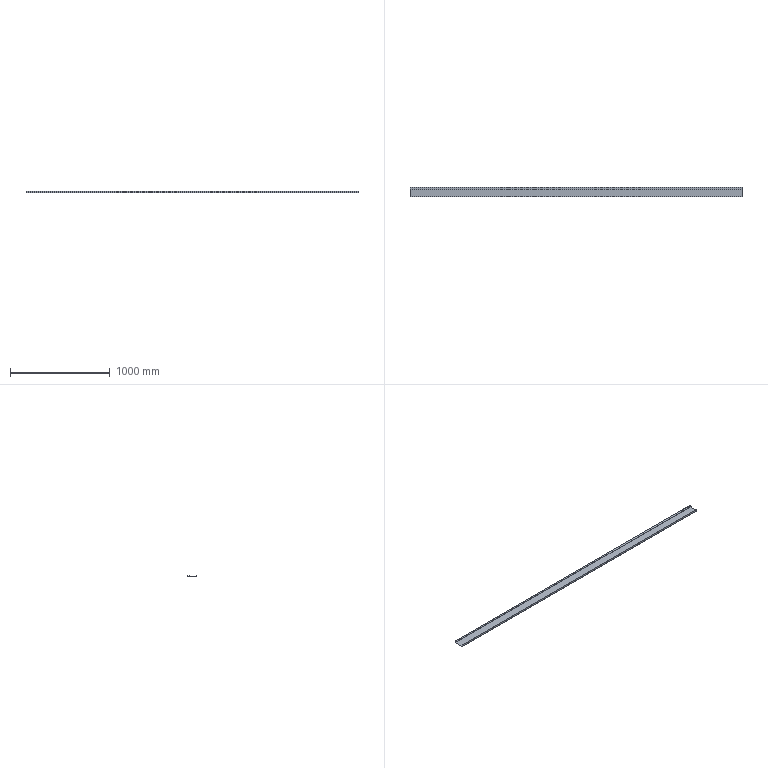Part | STEP file | 粉仓踢脚Plate 8 | 1 solid | 18 faces | box 3330 x 100 x 20 mm | volume 765467 mm3 | plane 12 | cylinder 6 | commonest cylinder face diameters 2 x3 5 x3
STEP:
#1=CARTESIAN_POINT('',(0.,0.,0.));
#2=DIRECTION('',(0.,0.,1.));
#3=DIRECTION('',(1.,0.,0.));
#4=AXIS2_PLACEMENT_3D('',#1,#2,#3);
#5=CARTESIAN_POINT('',(-1665.,1.5,2.5));
#6=VERTEX_POINT('',#5);
#7=CARTESIAN_POINT('',(-1665.,1.5,20.));
#8=VERTEX_POINT('',#7);
#9=CARTESIAN_POINT('',(-1665.,1.5,2.5));
#10=DIRECTION('',(0.,0.,1.));
#11=VECTOR('',#10,1.);
#12=LINE('',#9,#11);
#13=CARTESIAN_POINT('',(1665.,1.5,2.5));
#14=DIRECTION('',(0.,-1.,0.));
#15=DIRECTION('',(0.,0.,-1.));
#16=AXIS2_PLACEMENT_3D('',#13,#14,#15);
#17=PLANE('',#16);
#18=CARTESIAN_POINT('',(0.,-3330.));
#19=DIRECTION('',(-1.,0.));
#20=VECTOR('',#19,1.);
#21=LINE('',#18,#20);
#22=(GEOMETRIC_REPRESENTATION_CONTEXT(2)PARAMETRIC_REPRESENTATION_CONTEXT()REPRESENTATION_CONTEXT('',''));
#23=DEFINITIONAL_REPRESENTATION('',(#21),#22);
#24=PCURVE('',#17,#23);
#25=CARTESIAN_POINT('',(-1665.,2.5,2.5));
#26=DIRECTION('',(-1.,0.,0.));
#27=DIRECTION('',(0.,0.,1.));
#28=AXIS2_PLACEMENT_3D('',#25,#26,#27);
#29=PLANE('',#28);
#30=CARTESIAN_POINT('',(0.,-1.));
#31=DIRECTION('',(1.,0.));
#32=VECTOR('',#31,1.);
#33=LINE('',#30,#32);
#34=(GEOMETRIC_REPRESENTATION_CONTEXT(2)PARAMETRIC_REPRESENTATION_CONTEXT()REPRESENTATION_CONTEXT('',''));
#35=DEFINITIONAL_REPRESENTATION('',(#33),#34);
#36=PCURVE('',#29,#35);
#37=SURFACE_CURVE('',#12,(#24,#36),.PCURVE_S1.);
#38=EDGE_CURVE('',#6,#8,#37,.T.);
#39=ORIENTED_EDGE('',*,*,#38,.T.);
#40=CARTESIAN_POINT('',(1665.,1.5,20.));
#41=VERTEX_POINT('',#40);
#42=CARTESIAN_POINT('',(1665.,1.5,20.));
#43=DIRECTION('',(-1.,0.,0.));
#44=VECTOR('',#43,1.);
#45=LINE('',#42,#44);
#46=CARTESIAN_POINT('',(-17.5,0.));
#47=DIRECTION('',(0.,-1.));
#48=VECTOR('',#47,1.);
#49=LINE('',#46,#48);
#50=(GEOMETRIC_REPRESENTATION_CONTEXT(2)PARAMETRIC_REPRESENTATION_CONTEXT()REPRESENTATION_CONTEXT('',''));
#51=DEFINITIONAL_REPRESENTATION('',(#49),#50);
#52=PCURVE('',#17,#51);
#53=CARTESIAN_POINT('',(1665.,0.,20.));
#54=DIRECTION('',(0.,0.,1.));
#55=DIRECTION('',(1.,0.,0.));
#56=AXIS2_PLACEMENT_3D('',#53,#54,#55);
#57=PLANE('',#56);
#58=CARTESIAN_POINT('',(0.,1.5));
#59=DIRECTION('',(-1.,0.));
#60=VECTOR('',#59,1.);
#61=LINE('',#58,#60);
#62=(GEOMETRIC_REPRESENTATION_CONTEXT(2)PARAMETRIC_REPRESENTATION_CONTEXT()REPRESENTATION_CONTEXT('',''));
#63=DEFINITIONAL_REPRESENTATION('',(#61),#62);
#64=PCURVE('',#57,#63);
#65=SURFACE_CURVE('',#45,(#52,#64),.PCURVE_S1.);
#66=EDGE_CURVE('',#41,#8,#65,.T.);
#67=ORIENTED_EDGE('',*,*,#66,.F.);
#68=CARTESIAN_POINT('',(1665.,1.5,2.5));
#69=VERTEX_POINT('',#68);
#70=CARTESIAN_POINT('',(1665.,1.5,2.5));
#71=DIRECTION('',(0.,0.,1.));
#72=VECTOR('',#71,1.);
#73=LINE('',#70,#72);
#74=CARTESIAN_POINT('',(0.,0.));
#75=DIRECTION('',(-1.,0.));
#76=VECTOR('',#75,1.);
#77=LINE('',#74,#76);
#78=(GEOMETRIC_REPRESENTATION_CONTEXT(2)PARAMETRIC_REPRESENTATION_CONTEXT()REPRESENTATION_CONTEXT('',''));
#79=DEFINITIONAL_REPRESENTATION('',(#77),#78);
#80=PCURVE('',#17,#79);
#81=CARTESIAN_POINT('',(1665.,2.5,2.5));
#82=DIRECTION('',(-1.,0.,0.));
#83=DIRECTION('',(0.,0.,1.));
#84=AXIS2_PLACEMENT_3D('',#81,#82,#83);
#85=PLANE('',#84);
#86=CARTESIAN_POINT('',(0.,-1.));
#87=DIRECTION('',(1.,0.));
#88=VECTOR('',#87,1.);
#89=LINE('',#86,#88);
#90=(GEOMETRIC_REPRESENTATION_CONTEXT(2)PARAMETRIC_REPRESENTATION_CONTEXT()REPRESENTATION_CONTEXT('',''));
#91=DEFINITIONAL_REPRESENTATION('',(#89),#90);
#92=PCURVE('',#85,#91);
#93=SURFACE_CURVE('',#73,(#80,#92),.PCURVE_S1.);
#94=EDGE_CURVE('',#69,#41,#93,.T.);
#95=ORIENTED_EDGE('',*,*,#94,.F.);
#96=CARTESIAN_POINT('',(1665.,1.5,2.5));
#97=DIRECTION('',(-1.,0.,0.));
#98=VECTOR('',#97,1.);
#99=LINE('',#96,#98);
#100=CARTESIAN_POINT('',(0.,0.));
#101=DIRECTION('',(0.,-1.));
#102=VECTOR('',#101,1.);
#103=LINE('',#100,#102);
#104=(GEOMETRIC_REPRESENTATION_CONTEXT(2)PARAMETRIC_REPRESENTATION_CONTEXT()REPRESENTATION_CONTEXT('',''));
#105=DEFINITIONAL_REPRESENTATION('',(#103),#104);
#106=PCURVE('',#17,#105);
#107=CARTESIAN_POINT('',(1665.,2.5,2.5));
#108=DIRECTION('',(-1.,0.,0.));
#109=DIRECTION('',(0.,0.,1.));
#110=AXIS2_PLACEMENT_3D('',#107,#108,#109);
#111=CYLINDRICAL_SURFACE('',#110,1.);
#112=CARTESIAN_POINT('',(4.712,0.));
#113=DIRECTION('',(0.,1.));
#114=VECTOR('',#113,1.);
#115=LINE('',#112,#114);
#116=(GEOMETRIC_REPRESENTATION_CONTEXT(2)PARAMETRIC_REPRESENTATION_CONTEXT()REPRESENTATION_CONTEXT('',''));
#117=DEFINITIONAL_REPRESENTATION('',(#115),#116);
#118=PCURVE('',#111,#117);
#119=SURFACE_CURVE('',#99,(#106,#118),.PCURVE_S1.);
#120=EDGE_CURVE('',#69,#6,#119,.T.);
#121=ORIENTED_EDGE('',*,*,#120,.T.);
#122=EDGE_LOOP('',(#39,#67,#95,#121));
#123=FACE_BOUND('',#122,.T.);
#124=ADVANCED_FACE('',(#123),#17,.F.);
#125=CARTESIAN_POINT('',(-1665.,0.,20.));
#126=VERTEX_POINT('',#125);
#127=CARTESIAN_POINT('',(-1665.,0.,20.));
#128=DIRECTION('',(0.,1.,0.));
#129=VECTOR('',#128,1.);
#130=LINE('',#127,#129);
#131=CARTESIAN_POINT('',(-3330.,0.));
#132=DIRECTION('',(0.,1.));
#133=VECTOR('',#132,1.);
#134=LINE('',#131,#133);
#135=(GEOMETRIC_REPRESENTATION_CONTEXT(2)PARAMETRIC_REPRESENTATION_CONTEXT()REPRESENTATION_CONTEXT('',''));
#136=DEFINITIONAL_REPRESENTATION('',(#134),#135);
#137=PCURVE('',#57,#136);
#138=CARTESIAN_POINT('',(17.5,-2.5));
#139=DIRECTION('',(0.,1.));
#140=VECTOR('',#139,1.);
#141=LINE('',#138,#140);
#142=(GEOMETRIC_REPRESENTATION_CONTEXT(2)PARAMETRIC_REPRESENTATION_CONTEXT()REPRESENTATION_CONTEXT('',''));
#143=DEFINITIONAL_REPRESENTATION('',(#141),#142);
#144=PCURVE('',#29,#143);
#145=SURFACE_CURVE('',#130,(#137,#144),.PCURVE_S1.);
#146=EDGE_CURVE('',#126,#8,#145,.T.);
#147=ORIENTED_EDGE('',*,*,#146,.F.);
#148=CARTESIAN_POINT('',(1665.,0.,20.));
#149=VERTEX_POINT('',#148);
#150=CARTESIAN_POINT('',(1665.,0.,20.));
#151=DIRECTION('',(-1.,0.,0.));
#152=VECTOR('',#151,1.);
#153=LINE('',#150,#152);
#154=CARTESIAN_POINT('',(0.,0.));
#155=DIRECTION('',(-1.,0.));
#156=VECTOR('',#155,1.);
#157=LINE('',#154,#156);
#158=(GEOMETRIC_REPRESENTATION_CONTEXT(2)PARAMETRIC_REPRESENTATION_CONTEXT()REPRESENTATION_CONTEXT('',''));
#159=DEFINITIONAL_REPRESENTATION('',(#157),#158);
#160=PCURVE('',#57,#159);
#161=CARTESIAN_POINT('',(1665.,0.,2.5));
#162=DIRECTION('',(0.,-1.,0.));
#163=DIRECTION('',(0.,0.,-1.));
#164=AXIS2_PLACEMENT_3D('',#161,#162,#163);
#165=PLANE('',#164);
#166=CARTESIAN_POINT('',(-17.5,0.));
#167=DIRECTION('',(0.,-1.));
#168=VECTOR('',#167,1.);
#169=LINE('',#166,#168);
#170=(GEOMETRIC_REPRESENTATION_CONTEXT(2)PARAMETRIC_REPRESENTATION_CONTEXT()REPRESENTATION_CONTEXT('',''));
#171=DEFINITIONAL_REPRESENTATION('',(#169),#170);
#172=PCURVE('',#165,#171);
#173=SURFACE_CURVE('',#153,(#160,#172),.PCURVE_S1.);
#174=EDGE_CURVE('',#149,#126,#173,.T.);
#175=ORIENTED_EDGE('',*,*,#174,.F.);
#176=CARTESIAN_POINT('',(1665.,0.,20.));
#177=DIRECTION('',(0.,1.,0.));
#178=VECTOR('',#177,1.);
#179=LINE('',#176,#178);
#180=CARTESIAN_POINT('',(0.,0.));
#181=DIRECTION('',(0.,1.));
#182=VECTOR('',#181,1.);
#183=LINE('',#180,#182);
#184=(GEOMETRIC_REPRESENTATION_CONTEXT(2)PARAMETRIC_REPRESENTATION_CONTEXT()REPRESENTATION_CONTEXT('',''));
#185=DEFINITIONAL_REPRESENTATION('',(#183),#184);
#186=PCURVE('',#57,#185);
#187=CARTESIAN_POINT('',(17.5,-2.5));
#188=DIRECTION('',(0.,1.));
#189=VECTOR('',#188,1.);
#190=LINE('',#187,#189);
#191=(GEOMETRIC_REPRESENTATION_CONTEXT(2)PARAMETRIC_REPRESENTATION_CONTEXT()REPRESENTATION_CONTEXT('',''));
#192=DEFINITIONAL_REPRESENTATION('',(#190),#191);
#193=PCURVE('',#85,#192);
#194=SURFACE_CURVE('',#179,(#186,#193),.PCURVE_S1.);
#195=EDGE_CURVE('',#149,#41,#194,.T.);
#196=ORIENTED_EDGE('',*,*,#195,.T.);
#197=ORIENTED_EDGE('',*,*,#66,.T.);
#198=EDGE_LOOP('',(#147,#175,#196,#197));
#199=FACE_BOUND('',#198,.T.);
#200=ADVANCED_FACE('',(#199),#57,.T.);
#201=CARTESIAN_POINT('',(-1665.,0.,2.5));
#202=VERTEX_POINT('',#201);
#203=CARTESIAN_POINT('',(-1665.,0.,2.5));
#204=DIRECTION('',(0.,0.,1.));
#205=VECTOR('',#204,1.);
#206=LINE('',#203,#205);
#207=CARTESIAN_POINT('',(0.,-3330.));
#208=DIRECTION('',(-1.,0.));
#209=VECTOR('',#208,1.);
#210=LINE('',#207,#209);
#211=(GEOMETRIC_REPRESENTATION_CONTEXT(2)PARAMETRIC_REPRESENTATION_CONTEXT()REPRESENTATION_CONTEXT('',''));
#212=DEFINITIONAL_REPRESENTATION('',(#210),#211);
#213=PCURVE('',#165,#212);
#214=CARTESIAN_POINT('',(0.,-2.5));
#215=DIRECTION('',(1.,0.));
#216=VECTOR('',#215,1.);
#217=LINE('',#214,#216);
#218=(GEOMETRIC_REPRESENTATION_CONTEXT(2)PARAMETRIC_REPRESENTATION_CONTEXT()REPRESENTATION_CONTEXT('',''));
#219=DEFINITIONAL_REPRESENTATION('',(#217),#218);
#220=PCURVE('',#29,#219);
#221=SURFACE_CURVE('',#206,(#213,#220),.PCURVE_S1.);
#222=EDGE_CURVE('',#202,#126,#221,.T.);
#223=ORIENTED_EDGE('',*,*,#222,.F.);
#224=CARTESIAN_POINT('',(1665.,0.,2.5));
#225=VERTEX_POINT('',#224);
#226=CARTESIAN_POINT('',(1665.,0.,2.5));
#227=DIRECTION('',(-1.,0.,0.));
#228=VECTOR('',#227,1.);
#229=LINE('',#226,#228);
#230=CARTESIAN_POINT('',(0.,0.));
#231=DIRECTION('',(0.,-1.));
#232=VECTOR('',#231,1.);
#233=LINE('',#230,#232);
#234=(GEOMETRIC_REPRESENTATION_CONTEXT(2)PARAMETRIC_REPRESENTATION_CONTEXT()REPRESENTATION_CONTEXT('',''));
#235=DEFINITIONAL_REPRESENTATION('',(#233),#234);
#236=PCURVE('',#165,#235);
#237=CARTESIAN_POINT('',(1665.,2.5,2.5));
#238=DIRECTION('',(-1.,0.,0.));
#239=DIRECTION('',(0.,0.,1.));
#240=AXIS2_PLACEMENT_3D('',#237,#238,#239);
#241=CYLINDRICAL_SURFACE('',#240,2.5);
#242=CARTESIAN_POINT('',(4.712,0.));
#243=DIRECTION('',(0.,1.));
#244=VECTOR('',#243,1.);
#245=LINE('',#242,#244);
#246=(GEOMETRIC_REPRESENTATION_CONTEXT(2)PARAMETRIC_REPRESENTATION_CONTEXT()REPRESENTATION_CONTEXT('',''));
#247=DEFINITIONAL_REPRESENTATION('',(#245),#246);
#248=PCURVE('',#241,#247);
#249=SURFACE_CURVE('',#229,(#236,#248),.PCURVE_S1.);
#250=EDGE_CURVE('',#225,#202,#249,.T.);
#251=ORIENTED_EDGE('',*,*,#250,.F.);
#252=CARTESIAN_POINT('',(1665.,0.,2.5));
#253=DIRECTION('',(0.,0.,1.));
#254=VECTOR('',#253,1.);
#255=LINE('',#252,#254);
#256=CARTESIAN_POINT('',(0.,0.));
#257=DIRECTION('',(-1.,0.));
#258=VECTOR('',#257,1.);
#259=LINE('',#256,#258);
#260=(GEOMETRIC_REPRESENTATION_CONTEXT(2)PARAMETRIC_REPRESENTATION_CONTEXT()REPRESENTATION_CONTEXT('',''));
#261=DEFINITIONAL_REPRESENTATION('',(#259),#260);
#262=PCURVE('',#165,#261);
#263=CARTESIAN_POINT('',(0.,-2.5));
#264=DIRECTION('',(1.,0.));
#265=VECTOR('',#264,1.);
#266=LINE('',#263,#265);
#267=(GEOMETRIC_REPRESENTATION_CONTEXT(2)PARAMETRIC_REPRESENTATION_CONTEXT()REPRESENTATION_CONTEXT('',''));
#268=DEFINITIONAL_REPRESENTATION('',(#266),#267);
#269=PCURVE('',#85,#268);
#270=SURFACE_CURVE('',#255,(#262,#269),.PCURVE_S1.);
#271=EDGE_CURVE('',#225,#149,#270,.T.);
#272=ORIENTED_EDGE('',*,*,#271,.T.);
#273=ORIENTED_EDGE('',*,*,#174,.T.);
#274=EDGE_LOOP('',(#223,#251,#272,#273));
#275=FACE_BOUND('',#274,.T.);
#276=ADVANCED_FACE('',(#275),#165,.T.);
#277=CARTESIAN_POINT('',(-1665.,2.5,0.));
#278=VERTEX_POINT('',#277);
#279=CARTESIAN_POINT('',(-1665.,2.5,2.5));
#280=DIRECTION('',(-1.,0.,0.));
#281=DIRECTION('',(0.,0.,1.));
#282=AXIS2_PLACEMENT_3D('',#279,#280,#281);
#283=CIRCLE('',#282,2.5);
#284=CARTESIAN_POINT('',(0.,3330.));
#285=DIRECTION('',(1.,0.));
#286=VECTOR('',#285,1.);
#287=LINE('',#284,#286);
#288=(GEOMETRIC_REPRESENTATION_CONTEXT(2)PARAMETRIC_REPRESENTATION_CONTEXT()REPRESENTATION_CONTEXT('',''));
#289=DEFINITIONAL_REPRESENTATION('',(#287),#288);
#290=PCURVE('',#241,#289);
#291=CARTESIAN_POINT('',(0.,0.));
#292=DIRECTION('',(1.,0.));
#293=AXIS2_PLACEMENT_2D('',#291,#292);
#294=CIRCLE('',#293,2.5);
#295=(GEOMETRIC_REPRESENTATION_CONTEXT(2)PARAMETRIC_REPRESENTATION_CONTEXT()REPRESENTATION_CONTEXT('',''));
#296=DEFINITIONAL_REPRESENTATION('',(#294),#295);
#297=PCURVE('',#29,#296);
#298=SURFACE_CURVE('',#283,(#290,#297),.PCURVE_S1.);
#299=EDGE_CURVE('',#278,#202,#298,.T.);
#300=ORIENTED_EDGE('',*,*,#299,.F.);
#301=CARTESIAN_POINT('',(1665.,2.5,0.));
#302=VERTEX_POINT('',#301);
#303=CARTESIAN_POINT('',(1665.,2.5,0.));
#304=DIRECTION('',(-1.,0.,0.));
#305=VECTOR('',#304,1.);
#306=LINE('',#303,#305);
#307=CARTESIAN_POINT('',(3.142,0.));
#308=DIRECTION('',(0.,1.));
#309=VECTOR('',#308,1.);
#310=LINE('',#307,#309);
#311=(GEOMETRIC_REPRESENTATION_CONTEXT(2)PARAMETRIC_REPRESENTATION_CONTEXT()REPRESENTATION_CONTEXT('',''));
#312=DEFINITIONAL_REPRESENTATION('',(#310),#311);
#313=PCURVE('',#241,#312);
#314=CARTESIAN_POINT('',(1665.,2.5,0.));
#315=DIRECTION('',(0.,0.,-1.));
#316=DIRECTION('',(-1.,0.,0.));
#317=AXIS2_PLACEMENT_3D('',#314,#315,#316);
#318=PLANE('',#317);
#319=CARTESIAN_POINT('',(0.,0.));
#320=DIRECTION('',(1.,0.));
#321=VECTOR('',#320,1.);
#322=LINE('',#319,#321);
#323=(GEOMETRIC_REPRESENTATION_CONTEXT(2)PARAMETRIC_REPRESENTATION_CONTEXT()REPRESENTATION_CONTEXT('',''));
#324=DEFINITIONAL_REPRESENTATION('',(#322),#323);
#325=PCURVE('',#318,#324);
#326=SURFACE_CURVE('',#306,(#313,#325),.PCURVE_S1.);
#327=EDGE_CURVE('',#302,#278,#326,.T.);
#328=ORIENTED_EDGE('',*,*,#327,.F.);
#329=CARTESIAN_POINT('',(1665.,2.5,2.5));
#330=DIRECTION('',(-1.,0.,0.));
#331=DIRECTION('',(0.,0.,1.));
#332=AXIS2_PLACEMENT_3D('',#329,#330,#331);
#333=CIRCLE('',#332,2.5);
#334=CARTESIAN_POINT('',(0.,0.));
#335=DIRECTION('',(1.,0.));
#336=VECTOR('',#335,1.);
#337=LINE('',#334,#336);
#338=(GEOMETRIC_REPRESENTATION_CONTEXT(2)PARAMETRIC_REPRESENTATION_CONTEXT()REPRESENTATION_CONTEXT('',''));
#339=DEFINITIONAL_REPRESENTATION('',(#337),#338);
#340=PCURVE('',#241,#339);
#341=CARTESIAN_POINT('',(0.,0.));
#342=DIRECTION('',(1.,0.));
#343=AXIS2_PLACEMENT_2D('',#341,#342);
#344=CIRCLE('',#343,2.5);
#345=(GEOMETRIC_REPRESENTATION_CONTEXT(2)PARAMETRIC_REPRESENTATION_CONTEXT()REPRESENTATION_CONTEXT('',''));
#346=DEFINITIONAL_REPRESENTATION('',(#344),#345);
#347=PCURVE('',#85,#346);
#348=SURFACE_CURVE('',#333,(#340,#347),.PCURVE_S1.);
#349=EDGE_CURVE('',#302,#225,#348,.T.);
#350=ORIENTED_EDGE('',*,*,#349,.T.);
#351=ORIENTED_EDGE('',*,*,#250,.T.);
#352=EDGE_LOOP('',(#300,#328,#350,#351));
#353=FACE_BOUND('',#352,.T.);
#354=ADVANCED_FACE('',(#353),#241,.T.);
#355=CARTESIAN_POINT('',(-1665.,97.5,0.));
#356=VERTEX_POINT('',#355);
#357=CARTESIAN_POINT('',(-1665.,2.5,0.));
#358=DIRECTION('',(0.,-1.,0.));
#359=VECTOR('',#358,1.);
#360=LINE('',#357,#359);
#361=CARTESIAN_POINT('',(3330.,0.));
#362=DIRECTION('',(0.,-1.));
#363=VECTOR('',#362,1.);
#364=LINE('',#361,#363);
#365=(GEOMETRIC_REPRESENTATION_CONTEXT(2)PARAMETRIC_REPRESENTATION_CONTEXT()REPRESENTATION_CONTEXT('',''));
#366=DEFINITIONAL_REPRESENTATION('',(#364),#365);
#367=PCURVE('',#318,#366);
#368=CARTESIAN_POINT('',(-2.5,0.));
#369=DIRECTION('',(0.,-1.));
#370=VECTOR('',#369,1.);
#371=LINE('',#368,#370);
#372=(GEOMETRIC_REPRESENTATION_CONTEXT(2)PARAMETRIC_REPRESENTATION_CONTEXT()REPRESENTATION_CONTEXT('',''));
#373=DEFINITIONAL_REPRESENTATION('',(#371),#372);
#374=PCURVE('',#29,#373);
#375=SURFACE_CURVE('',#360,(#367,#374),.PCURVE_S1.);
#376=EDGE_CURVE('',#356,#278,#375,.T.);
#377=ORIENTED_EDGE('',*,*,#376,.F.);
#378=CARTESIAN_POINT('',(1665.,97.5,0.));
#379=VERTEX_POINT('',#378);
#380=CARTESIAN_POINT('',(1665.,97.5,0.));
#381=DIRECTION('',(-1.,0.,0.));
#382=VECTOR('',#381,1.);
#383=LINE('',#380,#382);
#384=CARTESIAN_POINT('',(0.,95.));
#385=DIRECTION('',(1.,0.));
#386=VECTOR('',#385,1.);
#387=LINE('',#384,#386);
#388=(GEOMETRIC_REPRESENTATION_CONTEXT(2)PARAMETRIC_REPRESENTATION_CONTEXT()REPRESENTATION_CONTEXT('',''));
#389=DEFINITIONAL_REPRESENTATION('',(#387),#388);
#390=PCURVE('',#318,#389);
#391=CARTESIAN_POINT('',(1665.,97.5,2.5));
#392=DIRECTION('',(-1.,0.,0.));
#393=DIRECTION('',(0.,0.,1.));
#394=AXIS2_PLACEMENT_3D('',#391,#392,#393);
#395=CYLINDRICAL_SURFACE('',#394,2.5);
#396=CARTESIAN_POINT('',(3.142,0.));
#397=DIRECTION('',(0.,1.));
#398=VECTOR('',#397,1.);
#399=LINE('',#396,#398);
#400=(GEOMETRIC_REPRESENTATION_CONTEXT(2)PARAMETRIC_REPRESENTATION_CONTEXT()REPRESENTATION_CONTEXT('',''));
#401=DEFINITIONAL_REPRESENTATION('',(#399),#400);
#402=PCURVE('',#395,#401);
#403=SURFACE_CURVE('',#383,(#390,#402),.PCURVE_S1.);
#404=EDGE_CURVE('',#379,#356,#403,.T.);
#405=ORIENTED_EDGE('',*,*,#404,.F.);
#406=CARTESIAN_POINT('',(1665.,2.5,0.));
#407=DIRECTION('',(0.,-1.,0.));
#408=VECTOR('',#407,1.);
#409=LINE('',#406,#408);
#410=CARTESIAN_POINT('',(0.,0.));
#411=DIRECTION('',(0.,-1.));
#412=VECTOR('',#411,1.);
#413=LINE('',#410,#412);
#414=(GEOMETRIC_REPRESENTATION_CONTEXT(2)PARAMETRIC_REPRESENTATION_CONTEXT()REPRESENTATION_CONTEXT('',''));
#415=DEFINITIONAL_REPRESENTATION('',(#413),#414);
#416=PCURVE('',#318,#415);
#417=CARTESIAN_POINT('',(-2.5,0.));
#418=DIRECTION('',(0.,-1.));
#419=VECTOR('',#418,1.);
#420=LINE('',#417,#419);
#421=(GEOMETRIC_REPRESENTATION_CONTEXT(2)PARAMETRIC_REPRESENTATION_CONTEXT()REPRESENTATION_CONTEXT('',''));
#422=DEFINITIONAL_REPRESENTATION('',(#420),#421);
#423=PCURVE('',#85,#422);
#424=SURFACE_CURVE('',#409,(#416,#423),.PCURVE_S1.);
#425=EDGE_CURVE('',#379,#302,#424,.T.);
#426=ORIENTED_EDGE('',*,*,#425,.T.);
#427=ORIENTED_EDGE('',*,*,#327,.T.);
#428=EDGE_LOOP('',(#377,#405,#426,#427));
#429=FACE_BOUND('',#428,.T.);
#430=ADVANCED_FACE('',(#429),#318,.T.);
#431=CARTESIAN_POINT('',(-1665.,100.,2.5));
#432=VERTEX_POINT('',#431);
#433=CARTESIAN_POINT('',(-1665.,97.5,2.5));
#434=DIRECTION('',(-1.,0.,0.));
#435=DIRECTION('',(0.,0.,-1.));
#436=AXIS2_PLACEMENT_3D('',#433,#434,#435);
#437=CIRCLE('',#436,2.5);
#438=CARTESIAN_POINT('',(-3.142,3330.));
#439=DIRECTION('',(1.,0.));
#440=VECTOR('',#439,1.);
#441=LINE('',#438,#440);
#442=(GEOMETRIC_REPRESENTATION_CONTEXT(2)PARAMETRIC_REPRESENTATION_CONTEXT()REPRESENTATION_CONTEXT('',''));
#443=DEFINITIONAL_REPRESENTATION('',(#441),#442);
#444=PCURVE('',#395,#443);
#445=CARTESIAN_POINT('',(0.,95.));
#446=DIRECTION('',(-1.,0.));
#447=AXIS2_PLACEMENT_2D('',#445,#446);
#448=CIRCLE('',#447,2.5);
#449=(GEOMETRIC_REPRESENTATION_CONTEXT(2)PARAMETRIC_REPRESENTATION_CONTEXT()REPRESENTATION_CONTEXT('',''));
#450=DEFINITIONAL_REPRESENTATION('',(#448),#449);
#451=PCURVE('',#29,#450);
#452=SURFACE_CURVE('',#437,(#444,#451),.PCURVE_S1.);
#453=EDGE_CURVE('',#432,#356,#452,.T.);
#454=ORIENTED_EDGE('',*,*,#453,.F.);
#455=CARTESIAN_POINT('',(1665.,100.,2.5));
#456=VERTEX_POINT('',#455);
#457=CARTESIAN_POINT('',(1665.,100.,2.5));
#458=DIRECTION('',(-1.,0.,0.));
#459=VECTOR('',#458,1.);
#460=LINE('',#457,#459);
#461=CARTESIAN_POINT('',(1.571,0.));
#462=DIRECTION('',(0.,1.));
#463=VECTOR('',#462,1.);
#464=LINE('',#461,#463);
#465=(GEOMETRIC_REPRESENTATION_CONTEXT(2)PARAMETRIC_REPRESENTATION_CONTEXT()REPRESENTATION_CONTEXT('',''));
#466=DEFINITIONAL_REPRESENTATION('',(#464),#465);
#467=PCURVE('',#395,#466);
#468=CARTESIAN_POINT('',(1665.,100.,2.5));
#469=DIRECTION('',(0.,1.,0.));
#470=DIRECTION('',(0.,0.,1.));
#471=AXIS2_PLACEMENT_3D('',#468,#469,#470);
#472=PLANE('',#471);
#473=CARTESIAN_POINT('',(0.,0.));
#474=DIRECTION('',(0.,-1.));
#475=VECTOR('',#474,1.);
#476=LINE('',#473,#475);
#477=(GEOMETRIC_REPRESENTATION_CONTEXT(2)PARAMETRIC_REPRESENTATION_CONTEXT()REPRESENTATION_CONTEXT('',''));
#478=DEFINITIONAL_REPRESENTATION('',(#476),#477);
#479=PCURVE('',#472,#478);
#480=SURFACE_CURVE('',#460,(#467,#479),.PCURVE_S1.);
#481=EDGE_CURVE('',#456,#432,#480,.T.);
#482=ORIENTED_EDGE('',*,*,#481,.F.);
#483=CARTESIAN_POINT('',(1665.,97.5,2.5));
#484=DIRECTION('',(-1.,0.,0.));
#485=DIRECTION('',(0.,0.,-1.));
#486=AXIS2_PLACEMENT_3D('',#483,#484,#485);
#487=CIRCLE('',#486,2.5);
#488=CARTESIAN_POINT('',(-3.142,0.));
#489=DIRECTION('',(1.,0.));
#490=VECTOR('',#489,1.);
#491=LINE('',#488,#490);
#492=(GEOMETRIC_REPRESENTATION_CONTEXT(2)PARAMETRIC_REPRESENTATION_CONTEXT()REPRESENTATION_CONTEXT('',''));
#493=DEFINITIONAL_REPRESENTATION('',(#491),#492);
#494=PCURVE('',#395,#493);
#495=CARTESIAN_POINT('',(0.,95.));
#496=DIRECTION('',(-1.,0.));
#497=AXIS2_PLACEMENT_2D('',#495,#496);
#498=CIRCLE('',#497,2.5);
#499=(GEOMETRIC_REPRESENTATION_CONTEXT(2)PARAMETRIC_REPRESENTATION_CONTEXT()REPRESENTATION_CONTEXT('',''));
#500=DEFINITIONAL_REPRESENTATION('',(#498),#499);
#501=PCURVE('',#85,#500);
#502=SURFACE_CURVE('',#487,(#494,#501),.PCURVE_S1.);
#503=EDGE_CURVE('',#456,#379,#502,.T.);
#504=ORIENTED_EDGE('',*,*,#503,.T.);
#505=ORIENTED_EDGE('',*,*,#404,.T.);
#506=EDGE_LOOP('',(#454,#482,#504,#505));
#507=FACE_BOUND('',#506,.T.);
#508=ADVANCED_FACE('',(#507),#395,.T.);
#509=CARTESIAN_POINT('',(-1665.,100.,17.5));
#510=VERTEX_POINT('',#509);
#511=CARTESIAN_POINT('',(-1665.,100.,2.5));
#512=DIRECTION('',(0.,0.,-1.));
#513=VECTOR('',#512,1.);
#514=LINE('',#511,#513);
#515=CARTESIAN_POINT('',(0.,-3330.));
#516=DIRECTION('',(-1.,0.));
#517=VECTOR('',#516,1.);
#518=LINE('',#515,#517);
#519=(GEOMETRIC_REPRESENTATION_CONTEXT(2)PARAMETRIC_REPRESENTATION_CONTEXT()REPRESENTATION_CONTEXT('',''));
#520=DEFINITIONAL_REPRESENTATION('',(#518),#519);
#521=PCURVE('',#472,#520);
#522=CARTESIAN_POINT('',(0.,97.5));
#523=DIRECTION('',(-1.,0.));
#524=VECTOR('',#523,1.);
#525=LINE('',#522,#524);
#526=(GEOMETRIC_REPRESENTATION_CONTEXT(2)PARAMETRIC_REPRESENTATION_CONTEXT()REPRESENTATION_CONTEXT('',''));
#527=DEFINITIONAL_REPRESENTATION('',(#525),#526);
#528=PCURVE('',#29,#527);
#529=SURFACE_CURVE('',#514,(#521,#528),.PCURVE_S1.);
#530=EDGE_CURVE('',#510,#432,#529,.T.);
#531=ORIENTED_EDGE('',*,*,#530,.F.);
#532=CARTESIAN_POINT('',(1665.,100.,17.5));
#533=VERTEX_POINT('',#532);
#534=CARTESIAN_POINT('',(1665.,100.,17.5));
#535=DIRECTION('',(-1.,0.,0.));
#536=VECTOR('',#535,1.);
#537=LINE('',#534,#536);
#538=CARTESIAN_POINT('',(15.,0.));
#539=DIRECTION('',(0.,-1.));
#540=VECTOR('',#539,1.);
#541=LINE('',#538,#540);
#542=(GEOMETRIC_REPRESENTATION_CONTEXT(2)PARAMETRIC_REPRESENTATION_CONTEXT()REPRESENTATION_CONTEXT('',''));
#543=DEFINITIONAL_REPRESENTATION('',(#541),#542);
#544=PCURVE('',#472,#543);
#545=CARTESIAN_POINT('',(1665.,97.5,17.5));
#546=DIRECTION('',(-1.,0.,0.));
#547=DIRECTION('',(0.,0.,1.));
#548=AXIS2_PLACEMENT_3D('',#545,#546,#547);
#549=CYLINDRICAL_SURFACE('',#548,2.5);
#550=CARTESIAN_POINT('',(1.571,0.));
#551=DIRECTION('',(0.,1.));
#552=VECTOR('',#551,1.);
#553=LINE('',#550,#552);
#554=(GEOMETRIC_REPRESENTATION_CONTEXT(2)PARAMETRIC_REPRESENTATION_CONTEXT()REPRESENTATION_CONTEXT('',''));
#555=DEFINITIONAL_REPRESENTATION('',(#553),#554);
#556=PCURVE('',#549,#555);
#557=SURFACE_CURVE('',#537,(#544,#556),.PCURVE_S1.);
#558=EDGE_CURVE('',#533,#510,#557,.T.);
#559=ORIENTED_EDGE('',*,*,#558,.F.);
#560=CARTESIAN_POINT('',(1665.,100.,2.5));
#561=DIRECTION('',(0.,0.,-1.));
#562=VECTOR('',#561,1.);
#563=LINE('',#560,#562);
#564=CARTESIAN_POINT('',(0.,0.));
#565=DIRECTION('',(-1.,0.));
#566=VECTOR('',#565,1.);
#567=LINE('',#564,#566);
#568=(GEOMETRIC_REPRESENTATION_CONTEXT(2)PARAMETRIC_REPRESENTATION_CONTEXT()REPRESENTATION_CONTEXT('',''));
#569=DEFINITIONAL_REPRESENTATION('',(#567),#568);
#570=PCURVE('',#472,#569);
#571=CARTESIAN_POINT('',(0.,97.5));
#572=DIRECTION('',(-1.,0.));
#573=VECTOR('',#572,1.);
#574=LINE('',#571,#573);
#575=(GEOMETRIC_REPRESENTATION_CONTEXT(2)PARAMETRIC_REPRESENTATION_CONTEXT()REPRESENTATION_CONTEXT('',''));
#576=DEFINITIONAL_REPRESENTATION('',(#574),#575);
#577=PCURVE('',#85,#576);
#578=SURFACE_CURVE('',#563,(#570,#577),.PCURVE_S1.);
#579=EDGE_CURVE('',#533,#456,#578,.T.);
#580=ORIENTED_EDGE('',*,*,#579,.T.);
#581=ORIENTED_EDGE('',*,*,#481,.T.);
#582=EDGE_LOOP('',(#531,#559,#580,#581));
#583=FACE_BOUND('',#582,.T.);
#584=ADVANCED_FACE('',(#583),#472,.T.);
#585=CARTESIAN_POINT('',(-1665.,97.5,20.));
#586=VERTEX_POINT('',#585);
#587=CARTESIAN_POINT('',(-1665.,97.5,17.5));
#588=DIRECTION('',(-1.,0.,0.));
#589=DIRECTION('',(0.,0.,-1.));
#590=AXIS2_PLACEMENT_3D('',#587,#588,#589);
#591=CIRCLE('',#590,2.5);
#592=CARTESIAN_POINT('',(-3.142,3330.));
#593=DIRECTION('',(1.,0.));
#594=VECTOR('',#593,1.);
#595=LINE('',#592,#594);
#596=(GEOMETRIC_REPRESENTATION_CONTEXT(2)PARAMETRIC_REPRESENTATION_CONTEXT()REPRESENTATION_CONTEXT('',''));
#597=DEFINITIONAL_REPRESENTATION('',(#595),#596);
#598=PCURVE('',#549,#597);
#599=CARTESIAN_POINT('',(15.,95.));
#600=DIRECTION('',(-1.,0.));
#601=AXIS2_PLACEMENT_2D('',#599,#600);
#602=CIRCLE('',#601,2.5);
#603=(GEOMETRIC_REPRESENTATION_CONTEXT(2)PARAMETRIC_REPRESENTATION_CONTEXT()REPRESENTATION_CONTEXT('',''));
#604=DEFINITIONAL_REPRESENTATION('',(#602),#603);
#605=PCURVE('',#29,#604);
#606=SURFACE_CURVE('',#591,(#598,#605),.PCURVE_S1.);
#607=EDGE_CURVE('',#586,#510,#606,.T.);
#608=ORIENTED_EDGE('',*,*,#607,.F.);
#609=CARTESIAN_POINT('',(1665.,97.5,20.));
#610=VERTEX_POINT('',#609);
#611=CARTESIAN_POINT('',(1665.,97.5,20.));
#612=DIRECTION('',(-1.,0.,0.));
#613=VECTOR('',#612,1.);
#614=LINE('',#611,#613);
#615=CARTESIAN_POINT('',(0.,0.));
#616=DIRECTION('',(0.,1.));
#617=VECTOR('',#616,1.);
#618=LINE('',#615,#617);
#619=(GEOMETRIC_REPRESENTATION_CONTEXT(2)PARAMETRIC_REPRESENTATION_CONTEXT()REPRESENTATION_CONTEXT('',''));
#620=DEFINITIONAL_REPRESENTATION('',(#618),#619);
#621=PCURVE('',#549,#620);
#622=CARTESIAN_POINT('',(1665.,97.5,20.));
#623=DIRECTION('',(0.,0.,1.));
#624=DIRECTION('',(1.,0.,0.));
#625=AXIS2_PLACEMENT_3D('',#622,#623,#624);
#626=PLANE('',#625);
#627=CARTESIAN_POINT('',(0.,0.));
#628=DIRECTION('',(-1.,0.));
#629=VECTOR('',#628,1.);
#630=LINE('',#627,#629);
#631=(GEOMETRIC_REPRESENTATION_CONTEXT(2)PARAMETRIC_REPRESENTATION_CONTEXT()REPRESENTATION_CONTEXT('',''));
#632=DEFINITIONAL_REPRESENTATION('',(#630),#631);
#633=PCURVE('',#626,#632);
#634=SURFACE_CURVE('',#614,(#621,#633),.PCURVE_S1.);
#635=EDGE_CURVE('',#610,#586,#634,.T.);
#636=ORIENTED_EDGE('',*,*,#635,.F.);
#637=CARTESIAN_POINT('',(1665.,97.5,17.5));
#638=DIRECTION('',(-1.,0.,0.));
#639=DIRECTION('',(0.,0.,-1.));
#640=AXIS2_PLACEMENT_3D('',#637,#638,#639);
#641=CIRCLE('',#640,2.5);
#642=CARTESIAN_POINT('',(-3.142,0.));
#643=DIRECTION('',(1.,0.));
#644=VECTOR('',#643,1.);
#645=LINE('',#642,#644);
#646=(GEOMETRIC_REPRESENTATION_CONTEXT(2)PARAMETRIC_REPRESENTATION_CONTEXT()REPRESENTATION_CONTEXT('',''));
#647=DEFINITIONAL_REPRESENTATION('',(#645),#646);
#648=PCURVE('',#549,#647);
#649=CARTESIAN_POINT('',(15.,95.));
#650=DIRECTION('',(-1.,0.));
#651=AXIS2_PLACEMENT_2D('',#649,#650);
#652=CIRCLE('',#651,2.5);
#653=(GEOMETRIC_REPRESENTATION_CONTEXT(2)PARAMETRIC_REPRESENTATION_CONTEXT()REPRESENTATION_CONTEXT('',''));
#654=DEFINITIONAL_REPRESENTATION('',(#652),#653);
#655=PCURVE('',#85,#654);
#656=SURFACE_CURVE('',#641,(#648,#655),.PCURVE_S1.);
#657=EDGE_CURVE('',#610,#533,#656,.T.);
#658=ORIENTED_EDGE('',*,*,#657,.T.);
#659=ORIENTED_EDGE('',*,*,#558,.T.);
#660=EDGE_LOOP('',(#608,#636,#658,#659));
#661=FACE_BOUND('',#660,.T.);
#662=ADVANCED_FACE('',(#661),#549,.T.);
#663=CARTESIAN_POINT('',(-1665.,80.,20.));
#664=VERTEX_POINT('',#663);
#665=CARTESIAN_POINT('',(-1665.,97.5,20.));
#666=DIRECTION('',(0.,1.,0.));
#667=VECTOR('',#666,1.);
#668=LINE('',#665,#667);
#669=CARTESIAN_POINT('',(-3330.,0.));
#670=DIRECTION('',(0.,1.));
#671=VECTOR('',#670,1.);
#672=LINE('',#669,#671);
#673=(GEOMETRIC_REPRESENTATION_CONTEXT(2)PARAMETRIC_REPRESENTATION_CONTEXT()REPRESENTATION_CONTEXT('',''));
#674=DEFINITIONAL_REPRESENTATION('',(#672),#673);
#675=PCURVE('',#626,#674);
#676=CARTESIAN_POINT('',(17.5,95.));
#677=DIRECTION('',(0.,1.));
#678=VECTOR('',#677,1.);
#679=LINE('',#676,#678);
#680=(GEOMETRIC_REPRESENTATION_CONTEXT(2)PARAMETRIC_REPRESENTATION_CONTEXT()REPRESENTATION_CONTEXT('',''));
#681=DEFINITIONAL_REPRESENTATION('',(#679),#680);
#682=PCURVE('',#29,#681);
#683=SURFACE_CURVE('',#668,(#675,#682),.PCURVE_S1.);
#684=EDGE_CURVE('',#664,#586,#683,.T.);
#685=ORIENTED_EDGE('',*,*,#684,.F.);
#686=CARTESIAN_POINT('',(1665.,80.,20.));
#687=VERTEX_POINT('',#686);
#688=CARTESIAN_POINT('',(1665.,80.,20.));
#689=DIRECTION('',(-1.,0.,0.));
#690=VECTOR('',#689,1.);
#691=LINE('',#688,#690);
#692=CARTESIAN_POINT('',(0.,-17.5));
#693=DIRECTION('',(-1.,0.));
#694=VECTOR('',#693,1.);
#695=LINE('',#692,#694);
#696=(GEOMETRIC_REPRESENTATION_CONTEXT(2)PARAMETRIC_REPRESENTATION_CONTEXT()REPRESENTATION_CONTEXT('',''));
#697=DEFINITIONAL_REPRESENTATION('',(#695),#696);
#698=PCURVE('',#626,#697);
#699=CARTESIAN_POINT('',(1665.,80.,18.5));
#700=DIRECTION('',(0.,-1.,0.));
#701=DIRECTION('',(0.,0.,-1.));
#702=AXIS2_PLACEMENT_3D('',#699,#700,#701);
#703=PLANE('',#702);
#704=CARTESIAN_POINT('',(-1.5,0.));
#705=DIRECTION('',(0.,-1.));
#706=VECTOR('',#705,1.);
#707=LINE('',#704,#706);
#708=(GEOMETRIC_REPRESENTATION_CONTEXT(2)PARAMETRIC_REPRESENTATION_CONTEXT()REPRESENTATION_CONTEXT('',''));
#709=DEFINITIONAL_REPRESENTATION('',(#707),#708);
#710=PCURVE('',#703,#709);
#711=SURFACE_CURVE('',#691,(#698,#710),.PCURVE_S1.);
#712=EDGE_CURVE('',#687,#664,#711,.T.);
#713=ORIENTED_EDGE('',*,*,#712,.F.);
#714=CARTESIAN_POINT('',(1665.,97.5,20.));
#715=DIRECTION('',(0.,1.,0.));
#716=VECTOR('',#715,1.);
#717=LINE('',#714,#716);
#718=CARTESIAN_POINT('',(0.,0.));
#719=DIRECTION('',(0.,1.));
#720=VECTOR('',#719,1.);
#721=LINE('',#718,#720);
#722=(GEOMETRIC_REPRESENTATION_CONTEXT(2)PARAMETRIC_REPRESENTATION_CONTEXT()REPRESENTATION_CONTEXT('',''));
#723=DEFINITIONAL_REPRESENTATION('',(#721),#722);
#724=PCURVE('',#626,#723);
#725=CARTESIAN_POINT('',(17.5,95.));
#726=DIRECTION('',(0.,1.));
#727=VECTOR('',#726,1.);
#728=LINE('',#725,#727);
#729=(GEOMETRIC_REPRESENTATION_CONTEXT(2)PARAMETRIC_REPRESENTATION_CONTEXT()REPRESENTATION_CONTEXT('',''));
#730=DEFINITIONAL_REPRESENTATION('',(#728),#729);
#731=PCURVE('',#85,#730);
#732=SURFACE_CURVE('',#717,(#724,#731),.PCURVE_S1.);
#733=EDGE_CURVE('',#687,#610,#732,.T.);
#734=ORIENTED_EDGE('',*,*,#733,.T.);
#735=ORIENTED_EDGE('',*,*,#635,.T.);
#736=EDGE_LOOP('',(#685,#713,#734,#735));
#737=FACE_BOUND('',#736,.T.);
#738=ADVANCED_FACE('',(#737),#626,.T.);
#739=CARTESIAN_POINT('',(-1665.,80.,18.5));
#740=VERTEX_POINT('',#739);
#741=CARTESIAN_POINT('',(-1665.,80.,18.5));
#742=DIRECTION('',(0.,0.,1.));
#743=VECTOR('',#742,1.);
#744=LINE('',#741,#743);
#745=CARTESIAN_POINT('',(0.,-3330.));
#746=DIRECTION('',(-1.,0.));
#747=VECTOR('',#746,1.);
#748=LINE('',#745,#747);
#749=(GEOMETRIC_REPRESENTATION_CONTEXT(2)PARAMETRIC_REPRESENTATION_CONTEXT()REPRESENTATION_CONTEXT('',''));
#750=DEFINITIONAL_REPRESENTATION('',(#748),#749);
#751=PCURVE('',#703,#750);
#752=CARTESIAN_POINT('',(16.,77.5));
#753=DIRECTION('',(1.,0.));
#754=VECTOR('',#753,1.);
#755=LINE('',#752,#754);
#756=(GEOMETRIC_REPRESENTATION_CONTEXT(2)PARAMETRIC_REPRESENTATION_CONTEXT()REPRESENTATION_CONTEXT('',''));
#757=DEFINITIONAL_REPRESENTATION('',(#755),#756);
#758=PCURVE('',#29,#757);
#759=SURFACE_CURVE('',#744,(#751,#758),.PCURVE_S1.);
#760=EDGE_CURVE('',#740,#664,#759,.T.);
#761=ORIENTED_EDGE('',*,*,#760,.F.);
#762=CARTESIAN_POINT('',(1665.,80.,18.5));
#763=VERTEX_POINT('',#762);
#764=CARTESIAN_POINT('',(1665.,80.,18.5));
#765=DIRECTION('',(-1.,0.,0.));
#766=VECTOR('',#765,1.);
#767=LINE('',#764,#766);
#768=CARTESIAN_POINT('',(0.,0.));
#769=DIRECTION('',(0.,-1.));
#770=VECTOR('',#769,1.);
#771=LINE('',#768,#770);
#772=(GEOMETRIC_REPRESENTATION_CONTEXT(2)PARAMETRIC_REPRESENTATION_CONTEXT()REPRESENTATION_CONTEXT('',''));
#773=DEFINITIONAL_REPRESENTATION('',(#771),#772);
#774=PCURVE('',#703,#773);
#775=CARTESIAN_POINT('',(1665.,97.5,18.5));
#776=DIRECTION('',(0.,0.,1.));
#777=DIRECTION('',(1.,0.,0.));
#778=AXIS2_PLACEMENT_3D('',#775,#776,#777);
#779=PLANE('',#778);
#780=CARTESIAN_POINT('',(0.,-17.5));
#781=DIRECTION('',(-1.,0.));
#782=VECTOR('',#781,1.);
#783=LINE('',#780,#782);
#784=(GEOMETRIC_REPRESENTATION_CONTEXT(2)PARAMETRIC_REPRESENTATION_CONTEXT()REPRESENTATION_CONTEXT('',''));
#785=DEFINITIONAL_REPRESENTATION('',(#783),#784);
#786=PCURVE('',#779,#785);
#787=SURFACE_CURVE('',#767,(#774,#786),.PCURVE_S1.);
#788=EDGE_CURVE('',#763,#740,#787,.T.);
#789=ORIENTED_EDGE('',*,*,#788,.F.);
#790=CARTESIAN_POINT('',(1665.,80.,18.5));
#791=DIRECTION('',(0.,0.,1.));
#792=VECTOR('',#791,1.);
#793=LINE('',#790,#792);
#794=CARTESIAN_POINT('',(0.,0.));
#795=DIRECTION('',(-1.,0.));
#796=VECTOR('',#795,1.);
#797=LINE('',#794,#796);
#798=(GEOMETRIC_REPRESENTATION_CONTEXT(2)PARAMETRIC_REPRESENTATION_CONTEXT()REPRESENTATION_CONTEXT('',''));
#799=DEFINITIONAL_REPRESENTATION('',(#797),#798);
#800=PCURVE('',#703,#799);
#801=CARTESIAN_POINT('',(16.,77.5));
#802=DIRECTION('',(1.,0.));
#803=VECTOR('',#802,1.);
#804=LINE('',#801,#803);
#805=(GEOMETRIC_REPRESENTATION_CONTEXT(2)PARAMETRIC_REPRESENTATION_CONTEXT()REPRESENTATION_CONTEXT('',''));
#806=DEFINITIONAL_REPRESENTATION('',(#804),#805);
#807=PCURVE('',#85,#806);
#808=SURFACE_CURVE('',#793,(#800,#807),.PCURVE_S1.);
#809=EDGE_CURVE('',#763,#687,#808,.T.);
#810=ORIENTED_EDGE('',*,*,#809,.T.);
#811=ORIENTED_EDGE('',*,*,#712,.T.);
#812=EDGE_LOOP('',(#761,#789,#810,#811));
#813=FACE_BOUND('',#812,.T.);
#814=ADVANCED_FACE('',(#813),#703,.T.);
#815=CARTESIAN_POINT('',(-1665.,97.5,18.5));
#816=VERTEX_POINT('',#815);
#817=CARTESIAN_POINT('',(-1665.,97.5,18.5));
#818=DIRECTION('',(0.,1.,0.));
#819=VECTOR('',#818,1.);
#820=LINE('',#817,#819);
#821=CARTESIAN_POINT('',(-3330.,0.));
#822=DIRECTION('',(0.,1.));
#823=VECTOR('',#822,1.);
#824=LINE('',#821,#823);
#825=(GEOMETRIC_REPRESENTATION_CONTEXT(2)PARAMETRIC_REPRESENTATION_CONTEXT()REPRESENTATION_CONTEXT('',''));
#826=DEFINITIONAL_REPRESENTATION('',(#824),#825);
#827=PCURVE('',#779,#826);
#828=CARTESIAN_POINT('',(16.,95.));
#829=DIRECTION('',(0.,1.));
#830=VECTOR('',#829,1.);
#831=LINE('',#828,#830);
#832=(GEOMETRIC_REPRESENTATION_CONTEXT(2)PARAMETRIC_REPRESENTATION_CONTEXT()REPRESENTATION_CONTEXT('',''));
#833=DEFINITIONAL_REPRESENTATION('',(#831),#832);
#834=PCURVE('',#29,#833);
#835=SURFACE_CURVE('',#820,(#827,#834),.PCURVE_S1.);
#836=EDGE_CURVE('',#740,#816,#835,.T.);
#837=ORIENTED_EDGE('',*,*,#836,.T.);
#838=CARTESIAN_POINT('',(1665.,97.5,18.5));
#839=VERTEX_POINT('',#838);
#840=CARTESIAN_POINT('',(1665.,97.5,18.5));
#841=DIRECTION('',(-1.,0.,0.));
#842=VECTOR('',#841,1.);
#843=LINE('',#840,#842);
#844=CARTESIAN_POINT('',(0.,0.));
#845=DIRECTION('',(-1.,0.));
#846=VECTOR('',#845,1.);
#847=LINE('',#844,#846);
#848=(GEOMETRIC_REPRESENTATION_CONTEXT(2)PARAMETRIC_REPRESENTATION_CONTEXT()REPRESENTATION_CONTEXT('',''));
#849=DEFINITIONAL_REPRESENTATION('',(#847),#848);
#850=PCURVE('',#779,#849);
#851=CARTESIAN_POINT('',(1665.,97.5,17.5));
#852=DIRECTION('',(-1.,0.,0.));
#853=DIRECTION('',(0.,0.,1.));
#854=AXIS2_PLACEMENT_3D('',#851,#852,#853);
#855=CYLINDRICAL_SURFACE('',#854,1.);
#856=CARTESIAN_POINT('',(0.,0.));
#857=DIRECTION('',(0.,1.));
#858=VECTOR('',#857,1.);
#859=LINE('',#856,#858);
#860=(GEOMETRIC_REPRESENTATION_CONTEXT(2)PARAMETRIC_REPRESENTATION_CONTEXT()REPRESENTATION_CONTEXT('',''));
#861=DEFINITIONAL_REPRESENTATION('',(#859),#860);
#862=PCURVE('',#855,#861);
#863=SURFACE_CURVE('',#843,(#850,#862),.PCURVE_S1.);
#864=EDGE_CURVE('',#839,#816,#863,.T.);
#865=ORIENTED_EDGE('',*,*,#864,.F.);
#866=CARTESIAN_POINT('',(1665.,97.5,18.5));
#867=DIRECTION('',(0.,1.,0.));
#868=VECTOR('',#867,1.);
#869=LINE('',#866,#868);
#870=CARTESIAN_POINT('',(0.,0.));
#871=DIRECTION('',(0.,1.));
#872=VECTOR('',#871,1.);
#873=LINE('',#870,#872);
#874=(GEOMETRIC_REPRESENTATION_CONTEXT(2)PARAMETRIC_REPRESENTATION_CONTEXT()REPRESENTATION_CONTEXT('',''));
#875=DEFINITIONAL_REPRESENTATION('',(#873),#874);
#876=PCURVE('',#779,#875);
#877=CARTESIAN_POINT('',(16.,95.));
#878=DIRECTION('',(0.,1.));
#879=VECTOR('',#878,1.);
#880=LINE('',#877,#879);
#881=(GEOMETRIC_REPRESENTATION_CONTEXT(2)PARAMETRIC_REPRESENTATION_CONTEXT()REPRESENTATION_CONTEXT('',''));
#882=DEFINITIONAL_REPRESENTATION('',(#880),#881);
#883=PCURVE('',#85,#882);
#884=SURFACE_CURVE('',#869,(#876,#883),.PCURVE_S1.);
#885=EDGE_CURVE('',#763,#839,#884,.T.);
#886=ORIENTED_EDGE('',*,*,#885,.F.);
#887=ORIENTED_EDGE('',*,*,#788,.T.);
#888=EDGE_LOOP('',(#837,#865,#886,#887));
#889=FACE_BOUND('',#888,.T.);
#890=ADVANCED_FACE('',(#889),#779,.F.);
#891=ORIENTED_EDGE('',*,*,#864,.F.);
#892=CARTESIAN_POINT('',(1665.,98.5,17.5));
#893=VERTEX_POINT('',#892);
#894=CARTESIAN_POINT('',(1665.,97.5,17.5));
#895=DIRECTION('',(-1.,0.,0.));
#896=DIRECTION('',(0.,0.,-1.));
#897=AXIS2_PLACEMENT_3D('',#894,#895,#896);
#898=CIRCLE('',#897,1.);
#899=CARTESIAN_POINT('',(-3.142,0.));
#900=DIRECTION('',(1.,0.));
#901=VECTOR('',#900,1.);
#902=LINE('',#899,#901);
#903=(GEOMETRIC_REPRESENTATION_CONTEXT(2)PARAMETRIC_REPRESENTATION_CONTEXT()REPRESENTATION_CONTEXT('',''));
#904=DEFINITIONAL_REPRESENTATION('',(#902),#903);
#905=PCURVE('',#855,#904);
#906=CARTESIAN_POINT('',(15.,95.));
#907=DIRECTION('',(-1.,0.));
#908=AXIS2_PLACEMENT_2D('',#906,#907);
#909=CIRCLE('',#908,1.);
#910=(GEOMETRIC_REPRESENTATION_CONTEXT(2)PARAMETRIC_REPRESENTATION_CONTEXT()REPRESENTATION_CONTEXT('',''));
#911=DEFINITIONAL_REPRESENTATION('',(#909),#910);
#912=PCURVE('',#85,#911);
#913=SURFACE_CURVE('',#898,(#905,#912),.PCURVE_S1.);
#914=EDGE_CURVE('',#839,#893,#913,.T.);
#915=ORIENTED_EDGE('',*,*,#914,.T.);
#916=CARTESIAN_POINT('',(-1665.,98.5,17.5));
#917=VERTEX_POINT('',#916);
#918=CARTESIAN_POINT('',(1665.,98.5,17.5));
#919=DIRECTION('',(-1.,0.,0.));
#920=VECTOR('',#919,1.);
#921=LINE('',#918,#920);
#922=CARTESIAN_POINT('',(1.571,0.));
#923=DIRECTION('',(0.,1.));
#924=VECTOR('',#923,1.);
#925=LINE('',#922,#924);
#926=(GEOMETRIC_REPRESENTATION_CONTEXT(2)PARAMETRIC_REPRESENTATION_CONTEXT()REPRESENTATION_CONTEXT('',''));
#927=DEFINITIONAL_REPRESENTATION('',(#925),#926);
#928=PCURVE('',#855,#927);
#929=CARTESIAN_POINT('',(1665.,98.5,2.5));
#930=DIRECTION('',(0.,1.,0.));
#931=DIRECTION('',(0.,0.,1.));
#932=AXIS2_PLACEMENT_3D('',#929,#930,#931);
#933=PLANE('',#932);
#934=CARTESIAN_POINT('',(15.,0.));
#935=DIRECTION('',(0.,-1.));
#936=VECTOR('',#935,1.);
#937=LINE('',#934,#936);
#938=(GEOMETRIC_REPRESENTATION_CONTEXT(2)PARAMETRIC_REPRESENTATION_CONTEXT()REPRESENTATION_CONTEXT('',''));
#939=DEFINITIONAL_REPRESENTATION('',(#937),#938);
#940=PCURVE('',#933,#939);
#941=SURFACE_CURVE('',#921,(#928,#940),.PCURVE_S1.);
#942=EDGE_CURVE('',#893,#917,#941,.T.);
#943=ORIENTED_EDGE('',*,*,#942,.T.);
#944=CARTESIAN_POINT('',(-1665.,97.5,17.5));
#945=DIRECTION('',(-1.,0.,0.));
#946=DIRECTION('',(0.,0.,-1.));
#947=AXIS2_PLACEMENT_3D('',#944,#945,#946);
#948=CIRCLE('',#947,1.);
#949=CARTESIAN_POINT('',(-3.142,3330.));
#950=DIRECTION('',(1.,0.));
#951=VECTOR('',#950,1.);
#952=LINE('',#949,#951);
#953=(GEOMETRIC_REPRESENTATION_CONTEXT(2)PARAMETRIC_REPRESENTATION_CONTEXT()REPRESENTATION_CONTEXT('',''));
#954=DEFINITIONAL_REPRESENTATION('',(#952),#953);
#955=PCURVE('',#855,#954);
#956=CARTESIAN_POINT('',(15.,95.));
#957=DIRECTION('',(-1.,0.));
#958=AXIS2_PLACEMENT_2D('',#956,#957);
#959=CIRCLE('',#958,1.);
#960=(GEOMETRIC_REPRESENTATION_CONTEXT(2)PARAMETRIC_REPRESENTATION_CONTEXT()REPRESENTATION_CONTEXT('',''));
#961=DEFINITIONAL_REPRESENTATION('',(#959),#960);
#962=PCURVE('',#29,#961);
#963=SURFACE_CURVE('',#948,(#955,#962),.PCURVE_S1.);
#964=EDGE_CURVE('',#816,#917,#963,.T.);
#965=ORIENTED_EDGE('',*,*,#964,.F.);
#966=EDGE_LOOP('',(#891,#915,#943,#965));
#967=FACE_BOUND('',#966,.F.);
#968=ADVANCED_FACE('',(#967),#855,.F.);
#969=CARTESIAN_POINT('',(-1665.,98.5,2.5));
#970=VERTEX_POINT('',#969);
#971=CARTESIAN_POINT('',(-1665.,98.5,2.5));
#972=DIRECTION('',(0.,0.,-1.));
#973=VECTOR('',#972,1.);
#974=LINE('',#971,#973);
#975=CARTESIAN_POINT('',(0.,-3330.));
#976=DIRECTION('',(-1.,0.));
#977=VECTOR('',#976,1.);
#978=LINE('',#975,#977);
#979=(GEOMETRIC_REPRESENTATION_CONTEXT(2)PARAMETRIC_REPRESENTATION_CONTEXT()REPRESENTATION_CONTEXT('',''));
#980=DEFINITIONAL_REPRESENTATION('',(#978),#979);
#981=PCURVE('',#933,#980);
#982=CARTESIAN_POINT('',(0.,96.));
#983=DIRECTION('',(-1.,0.));
#984=VECTOR('',#983,1.);
#985=LINE('',#982,#984);
#986=(GEOMETRIC_REPRESENTATION_CONTEXT(2)PARAMETRIC_REPRESENTATION_CONTEXT()REPRESENTATION_CONTEXT('',''));
#987=DEFINITIONAL_REPRESENTATION('',(#985),#986);
#988=PCURVE('',#29,#987);
#989=SURFACE_CURVE('',#974,(#981,#988),.PCURVE_S1.);
#990=EDGE_CURVE('',#917,#970,#989,.T.);
#991=ORIENTED_EDGE('',*,*,#990,.T.);
#992=CARTESIAN_POINT('',(1665.,98.5,2.5));
#993=VERTEX_POINT('',#992);
#994=CARTESIAN_POINT('',(1665.,98.5,2.5));
#995=DIRECTION('',(-1.,0.,0.));
#996=VECTOR('',#995,1.);
#997=LINE('',#994,#996);
#998=CARTESIAN_POINT('',(0.,0.));
#999=DIRECTION('',(0.,-1.));
#1000=VECTOR('',#999,1.);
#1001=LINE('',#998,#1000);
#1002=(GEOMETRIC_REPRESENTATION_CONTEXT(2)PARAMETRIC_REPRESENTATION_CONTEXT()REPRESENTATION_CONTEXT('',''));
#1003=DEFINITIONAL_REPRESENTATION('',(#1001),#1002);
#1004=PCURVE('',#933,#1003);
#1005=CARTESIAN_POINT('',(1665.,97.5,2.5));
#1006=DIRECTION('',(-1.,0.,0.));
#1007=DIRECTION('',(0.,0.,1.));
#1008=AXIS2_PLACEMENT_3D('',#1005,#1006,#1007);
#1009=CYLINDRICAL_SURFACE('',#1008,1.);
#1010=CARTESIAN_POINT('',(1.571,0.));
#1011=DIRECTION('',(0.,1.));
#1012=VECTOR('',#1011,1.);
#1013=LINE('',#1010,#1012);
#1014=(GEOMETRIC_REPRESENTATION_CONTEXT(2)PARAMETRIC_REPRESENTATION_CONTEXT()REPRESENTATION_CONTEXT('',''));
#1015=DEFINITIONAL_REPRESENTATION('',(#1013),#1014);
#1016=PCURVE('',#1009,#1015);
#1017=SURFACE_CURVE('',#997,(#1004,#1016),.PCURVE_S1.);
#1018=EDGE_CURVE('',#993,#970,#1017,.T.);
#1019=ORIENTED_EDGE('',*,*,#1018,.F.);
#1020=CARTESIAN_POINT('',(1665.,98.5,2.5));
#1021=DIRECTION('',(0.,0.,-1.));
#1022=VECTOR('',#1021,1.);
#1023=LINE('',#1020,#1022);
#1024=CARTESIAN_POINT('',(0.,0.));
#1025=DIRECTION('',(-1.,0.));
#1026=VECTOR('',#1025,1.);
#1027=LINE('',#1024,#1026);
#1028=(GEOMETRIC_REPRESENTATION_CONTEXT(2)PARAMETRIC_REPRESENTATION_CONTEXT()REPRESENTATION_CONTEXT('',''));
#1029=DEFINITIONAL_REPRESENTATION('',(#1027),#1028);
#1030=PCURVE('',#933,#1029);
#1031=CARTESIAN_POINT('',(0.,96.));
#1032=DIRECTION('',(-1.,0.));
#1033=VECTOR('',#1032,1.);
#1034=LINE('',#1031,#1033);
#1035=(GEOMETRIC_REPRESENTATION_CONTEXT(2)PARAMETRIC_REPRESENTATION_CONTEXT()REPRESENTATION_CONTEXT('',''));
#1036=DEFINITIONAL_REPRESENTATION('',(#1034),#1035);
#1037=PCURVE('',#85,#1036);
#1038=SURFACE_CURVE('',#1023,(#1030,#1037),.PCURVE_S1.);
#1039=EDGE_CURVE('',#893,#993,#1038,.T.);
#1040=ORIENTED_EDGE('',*,*,#1039,.F.);
#1041=ORIENTED_EDGE('',*,*,#942,.T.);
#1042=EDGE_LOOP('',(#991,#1019,#1040,#1041));
#1043=FACE_BOUND('',#1042,.T.);
#1044=ADVANCED_FACE('',(#1043),#933,.F.);
#1045=ORIENTED_EDGE('',*,*,#1018,.F.);
#1046=CARTESIAN_POINT('',(1665.,97.5,1.5));
#1047=VERTEX_POINT('',#1046);
#1048=CARTESIAN_POINT('',(1665.,97.5,2.5));
#1049=DIRECTION('',(-1.,0.,0.));
#1050=DIRECTION('',(0.,0.,-1.));
#1051=AXIS2_PLACEMENT_3D('',#1048,#1049,#1050);
#1052=CIRCLE('',#1051,1.);
#1053=CARTESIAN_POINT('',(-3.142,0.));
#1054=DIRECTION('',(1.,0.));
#1055=VECTOR('',#1054,1.);
#1056=LINE('',#1053,#1055);
#1057=(GEOMETRIC_REPRESENTATION_CONTEXT(2)PARAMETRIC_REPRESENTATION_CONTEXT()REPRESENTATION_CONTEXT('',''));
#1058=DEFINITIONAL_REPRESENTATION('',(#1056),#1057);
#1059=PCURVE('',#1009,#1058);
#1060=CARTESIAN_POINT('',(0.,95.));
#1061=DIRECTION('',(-1.,0.));
#1062=AXIS2_PLACEMENT_2D('',#1060,#1061);
#1063=CIRCLE('',#1062,1.);
#1064=(GEOMETRIC_REPRESENTATION_CONTEXT(2)PARAMETRIC_REPRESENTATION_CONTEXT()REPRESENTATION_CONTEXT('',''));
#1065=DEFINITIONAL_REPRESENTATION('',(#1063),#1064);
#1066=PCURVE('',#85,#1065);
#1067=SURFACE_CURVE('',#1052,(#1059,#1066),.PCURVE_S1.);
#1068=EDGE_CURVE('',#993,#1047,#1067,.T.);
#1069=ORIENTED_EDGE('',*,*,#1068,.T.);
#1070=CARTESIAN_POINT('',(-1665.,97.5,1.5));
#1071=VERTEX_POINT('',#1070);
#1072=CARTESIAN_POINT('',(1665.,97.5,1.5));
#1073=DIRECTION('',(-1.,0.,0.));
#1074=VECTOR('',#1073,1.);
#1075=LINE('',#1072,#1074);
#1076=CARTESIAN_POINT('',(3.142,0.));
#1077=DIRECTION('',(0.,1.));
#1078=VECTOR('',#1077,1.);
#1079=LINE('',#1076,#1078);
#1080=(GEOMETRIC_REPRESENTATION_CONTEXT(2)PARAMETRIC_REPRESENTATION_CONTEXT()REPRESENTATION_CONTEXT('',''));
#1081=DEFINITIONAL_REPRESENTATION('',(#1079),#1080);
#1082=PCURVE('',#1009,#1081);
#1083=CARTESIAN_POINT('',(1665.,2.5,1.5));
#1084=DIRECTION('',(0.,0.,-1.));
#1085=DIRECTION('',(-1.,0.,0.));
#1086=AXIS2_PLACEMENT_3D('',#1083,#1084,#1085);
#1087=PLANE('',#1086);
#1088=CARTESIAN_POINT('',(0.,95.));
#1089=DIRECTION('',(1.,0.));
#1090=VECTOR('',#1089,1.);
#1091=LINE('',#1088,#1090);
#1092=(GEOMETRIC_REPRESENTATION_CONTEXT(2)PARAMETRIC_REPRESENTATION_CONTEXT()REPRESENTATION_CONTEXT('',''));
#1093=DEFINITIONAL_REPRESENTATION('',(#1091),#1092);
#1094=PCURVE('',#1087,#1093);
#1095=SURFACE_CURVE('',#1075,(#1082,#1094),.PCURVE_S1.);
#1096=EDGE_CURVE('',#1047,#1071,#1095,.T.);
#1097=ORIENTED_EDGE('',*,*,#1096,.T.);
#1098=CARTESIAN_POINT('',(-1665.,97.5,2.5));
#1099=DIRECTION('',(-1.,0.,0.));
#1100=DIRECTION('',(0.,0.,-1.));
#1101=AXIS2_PLACEMENT_3D('',#1098,#1099,#1100);
#1102=CIRCLE('',#1101,1.);
#1103=CARTESIAN_POINT('',(-3.142,3330.));
#1104=DIRECTION('',(1.,0.));
#1105=VECTOR('',#1104,1.);
#1106=LINE('',#1103,#1105);
#1107=(GEOMETRIC_REPRESENTATION_CONTEXT(2)PARAMETRIC_REPRESENTATION_CONTEXT()REPRESENTATION_CONTEXT('',''));
#1108=DEFINITIONAL_REPRESENTATION('',(#1106),#1107);
#1109=PCURVE('',#1009,#1108);
#1110=CARTESIAN_POINT('',(0.,95.));
#1111=DIRECTION('',(-1.,0.));
#1112=AXIS2_PLACEMENT_2D('',#1110,#1111);
#1113=CIRCLE('',#1112,1.);
#1114=(GEOMETRIC_REPRESENTATION_CONTEXT(2)PARAMETRIC_REPRESENTATION_CONTEXT()REPRESENTATION_CONTEXT('',''));
#1115=DEFINITIONAL_REPRESENTATION('',(#1113),#1114);
#1116=PCURVE('',#29,#1115);
#1117=SURFACE_CURVE('',#1102,(#1109,#1116),.PCURVE_S1.);
#1118=EDGE_CURVE('',#970,#1071,#1117,.T.);
#1119=ORIENTED_EDGE('',*,*,#1118,.F.);
#1120=EDGE_LOOP('',(#1045,#1069,#1097,#1119));
#1121=FACE_BOUND('',#1120,.F.);
#1122=ADVANCED_FACE('',(#1121),#1009,.F.);
#1123=CARTESIAN_POINT('',(-1665.,2.5,1.5));
#1124=VERTEX_POINT('',#1123);
#1125=CARTESIAN_POINT('',(-1665.,2.5,1.5));
#1126=DIRECTION('',(0.,-1.,0.));
#1127=VECTOR('',#1126,1.);
#1128=LINE('',#1125,#1127);
#1129=CARTESIAN_POINT('',(3330.,0.));
#1130=DIRECTION('',(0.,-1.));
#1131=VECTOR('',#1130,1.);
#1132=LINE('',#1129,#1131);
#1133=(GEOMETRIC_REPRESENTATION_CONTEXT(2)PARAMETRIC_REPRESENTATION_CONTEXT()REPRESENTATION_CONTEXT('',''));
#1134=DEFINITIONAL_REPRESENTATION('',(#1132),#1133);
#1135=PCURVE('',#1087,#1134);
#1136=CARTESIAN_POINT('',(-1.,0.));
#1137=DIRECTION('',(0.,-1.));
#1138=VECTOR('',#1137,1.);
#1139=LINE('',#1136,#1138);
#1140=(GEOMETRIC_REPRESENTATION_CONTEXT(2)PARAMETRIC_REPRESENTATION_CONTEXT()REPRESENTATION_CONTEXT('',''));
#1141=DEFINITIONAL_REPRESENTATION('',(#1139),#1140);
#1142=PCURVE('',#29,#1141);
#1143=SURFACE_CURVE('',#1128,(#1135,#1142),.PCURVE_S1.);
#1144=EDGE_CURVE('',#1071,#1124,#1143,.T.);
#1145=ORIENTED_EDGE('',*,*,#1144,.T.);
#1146=CARTESIAN_POINT('',(1665.,2.5,1.5));
#1147=VERTEX_POINT('',#1146);
#1148=CARTESIAN_POINT('',(1665.,2.5,1.5));
#1149=DIRECTION('',(-1.,0.,0.));
#1150=VECTOR('',#1149,1.);
#1151=LINE('',#1148,#1150);
#1152=CARTESIAN_POINT('',(0.,0.));
#1153=DIRECTION('',(1.,0.));
#1154=VECTOR('',#1153,1.);
#1155=LINE('',#1152,#1154);
#1156=(GEOMETRIC_REPRESENTATION_CONTEXT(2)PARAMETRIC_REPRESENTATION_CONTEXT()REPRESENTATION_CONTEXT('',''));
#1157=DEFINITIONAL_REPRESENTATION('',(#1155),#1156);
#1158=PCURVE('',#1087,#1157);
#1159=CARTESIAN_POINT('',(3.142,0.));
#1160=DIRECTION('',(0.,1.));
#1161=VECTOR('',#1160,1.);
#1162=LINE('',#1159,#1161);
#1163=(GEOMETRIC_REPRESENTATION_CONTEXT(2)PARAMETRIC_REPRESENTATION_CONTEXT()REPRESENTATION_CONTEXT('',''));
#1164=DEFINITIONAL_REPRESENTATION('',(#1162),#1163);
#1165=PCURVE('',#111,#1164);
#1166=SURFACE_CURVE('',#1151,(#1158,#1165),.PCURVE_S1.);
#1167=EDGE_CURVE('',#1147,#1124,#1166,.T.);
#1168=ORIENTED_EDGE('',*,*,#1167,.F.);
#1169=CARTESIAN_POINT('',(1665.,2.5,1.5));
#1170=DIRECTION('',(0.,-1.,0.));
#1171=VECTOR('',#1170,1.);
#1172=LINE('',#1169,#1171);
#1173=CARTESIAN_POINT('',(0.,0.));
#1174=DIRECTION('',(0.,-1.));
#1175=VECTOR('',#1174,1.);
#1176=LINE('',#1173,#1175);
#1177=(GEOMETRIC_REPRESENTATION_CONTEXT(2)PARAMETRIC_REPRESENTATION_CONTEXT()REPRESENTATION_CONTEXT('',''));
#1178=DEFINITIONAL_REPRESENTATION('',(#1176),#1177);
#1179=PCURVE('',#1087,#1178);
#1180=CARTESIAN_POINT('',(-1.,0.));
#1181=DIRECTION('',(0.,-1.));
#1182=VECTOR('',#1181,1.);
#1183=LINE('',#1180,#1182);
#1184=(GEOMETRIC_REPRESENTATION_CONTEXT(2)PARAMETRIC_REPRESENTATION_CONTEXT()REPRESENTATION_CONTEXT('',''));
#1185=DEFINITIONAL_REPRESENTATION('',(#1183),#1184);
#1186=PCURVE('',#85,#1185);
#1187=SURFACE_CURVE('',#1172,(#1179,#1186),.PCURVE_S1.);
#1188=EDGE_CURVE('',#1047,#1147,#1187,.T.);
#1189=ORIENTED_EDGE('',*,*,#1188,.F.);
#1190=ORIENTED_EDGE('',*,*,#1096,.T.);
#1191=EDGE_LOOP('',(#1145,#1168,#1189,#1190));
#1192=FACE_BOUND('',#1191,.T.);
#1193=ADVANCED_FACE('',(#1192),#1087,.F.);
#1194=ORIENTED_EDGE('',*,*,#1167,.F.);
#1195=CARTESIAN_POINT('',(1665.,2.5,2.5));
#1196=DIRECTION('',(-1.,0.,0.));
#1197=DIRECTION('',(0.,0.,-1.));
#1198=AXIS2_PLACEMENT_3D('',#1195,#1196,#1197);
#1199=CIRCLE('',#1198,1.);
#1200=CARTESIAN_POINT('',(3.142,0.));
#1201=DIRECTION('',(1.,0.));
#1202=VECTOR('',#1201,1.);
#1203=LINE('',#1200,#1202);
#1204=(GEOMETRIC_REPRESENTATION_CONTEXT(2)PARAMETRIC_REPRESENTATION_CONTEXT()REPRESENTATION_CONTEXT('',''));
#1205=DEFINITIONAL_REPRESENTATION('',(#1203),#1204);
#1206=PCURVE('',#111,#1205);
#1207=CARTESIAN_POINT('',(0.,0.));
#1208=DIRECTION('',(-1.,0.));
#1209=AXIS2_PLACEMENT_2D('',#1207,#1208);
#1210=CIRCLE('',#1209,1.);
#1211=(GEOMETRIC_REPRESENTATION_CONTEXT(2)PARAMETRIC_REPRESENTATION_CONTEXT()REPRESENTATION_CONTEXT('',''));
#1212=DEFINITIONAL_REPRESENTATION('',(#1210),#1211);
#1213=PCURVE('',#85,#1212);
#1214=SURFACE_CURVE('',#1199,(#1206,#1213),.PCURVE_S1.);
#1215=EDGE_CURVE('',#1147,#69,#1214,.T.);
#1216=ORIENTED_EDGE('',*,*,#1215,.T.);
#1217=ORIENTED_EDGE('',*,*,#120,.T.);
#1218=CARTESIAN_POINT('',(-1665.,2.5,2.5));
#1219=DIRECTION('',(-1.,0.,0.));
#1220=DIRECTION('',(0.,0.,-1.));
#1221=AXIS2_PLACEMENT_3D('',#1218,#1219,#1220);
#1222=CIRCLE('',#1221,1.);
#1223=CARTESIAN_POINT('',(3.142,3330.));
#1224=DIRECTION('',(1.,0.));
#1225=VECTOR('',#1224,1.);
#1226=LINE('',#1223,#1225);
#1227=(GEOMETRIC_REPRESENTATION_CONTEXT(2)PARAMETRIC_REPRESENTATION_CONTEXT()REPRESENTATION_CONTEXT('',''));
#1228=DEFINITIONAL_REPRESENTATION('',(#1226),#1227);
#1229=PCURVE('',#111,#1228);
#1230=CARTESIAN_POINT('',(0.,0.));
#1231=DIRECTION('',(-1.,0.));
#1232=AXIS2_PLACEMENT_2D('',#1230,#1231);
#1233=CIRCLE('',#1232,1.);
#1234=(GEOMETRIC_REPRESENTATION_CONTEXT(2)PARAMETRIC_REPRESENTATION_CONTEXT()REPRESENTATION_CONTEXT('',''));
#1235=DEFINITIONAL_REPRESENTATION('',(#1233),#1234);
#1236=PCURVE('',#29,#1235);
#1237=SURFACE_CURVE('',#1222,(#1229,#1236),.PCURVE_S1.);
#1238=EDGE_CURVE('',#1124,#6,#1237,.T.);
#1239=ORIENTED_EDGE('',*,*,#1238,.F.);
#1240=EDGE_LOOP('',(#1194,#1216,#1217,#1239));
#1241=FACE_BOUND('',#1240,.F.);
#1242=ADVANCED_FACE('',(#1241),#111,.F.);
#1243=ORIENTED_EDGE('',*,*,#94,.T.);
#1244=ORIENTED_EDGE('',*,*,#195,.F.);
#1245=ORIENTED_EDGE('',*,*,#271,.F.);
#1246=ORIENTED_EDGE('',*,*,#349,.F.);
#1247=ORIENTED_EDGE('',*,*,#425,.F.);
#1248=ORIENTED_EDGE('',*,*,#503,.F.);
#1249=ORIENTED_EDGE('',*,*,#579,.F.);
#1250=ORIENTED_EDGE('',*,*,#657,.F.);
#1251=ORIENTED_EDGE('',*,*,#733,.F.);
#1252=ORIENTED_EDGE('',*,*,#809,.F.);
#1253=ORIENTED_EDGE('',*,*,#885,.T.);
#1254=ORIENTED_EDGE('',*,*,#914,.T.);
#1255=ORIENTED_EDGE('',*,*,#1039,.T.);
#1256=ORIENTED_EDGE('',*,*,#1068,.T.);
#1257=ORIENTED_EDGE('',*,*,#1188,.T.);
#1258=ORIENTED_EDGE('',*,*,#1215,.T.);
#1259=EDGE_LOOP('',(#1243,#1244,#1245,#1246,#1247,#1248,#1249,#1250,#1251,#1252,#1253,#1254,#1255,#1256,#1257,#1258));
#1260=FACE_BOUND('',#1259,.T.);
#1261=ADVANCED_FACE('',(#1260),#85,.F.);
#1262=ORIENTED_EDGE('',*,*,#38,.F.);
#1263=ORIENTED_EDGE('',*,*,#1238,.F.);
#1264=ORIENTED_EDGE('',*,*,#1144,.F.);
#1265=ORIENTED_EDGE('',*,*,#1118,.F.);
#1266=ORIENTED_EDGE('',*,*,#990,.F.);
#1267=ORIENTED_EDGE('',*,*,#964,.F.);
#1268=ORIENTED_EDGE('',*,*,#836,.F.);
#1269=ORIENTED_EDGE('',*,*,#760,.T.);
#1270=ORIENTED_EDGE('',*,*,#684,.T.);
#1271=ORIENTED_EDGE('',*,*,#607,.T.);
#1272=ORIENTED_EDGE('',*,*,#530,.T.);
#1273=ORIENTED_EDGE('',*,*,#453,.T.);
#1274=ORIENTED_EDGE('',*,*,#376,.T.);
#1275=ORIENTED_EDGE('',*,*,#299,.T.);
#1276=ORIENTED_EDGE('',*,*,#222,.T.);
#1277=ORIENTED_EDGE('',*,*,#146,.T.);
#1278=EDGE_LOOP('',(#1262,#1263,#1264,#1265,#1266,#1267,#1268,#1269,#1270,#1271,#1272,#1273,#1274,#1275,#1276,#1277));
#1279=FACE_BOUND('',#1278,.T.);
#1280=ADVANCED_FACE('',(#1279),#29,.T.);
#1281=CLOSED_SHELL('',(#124,#200,#276,#354,#430,#508,#584,#662,#738,#814,#890,#968,#1044,#1122,#1193,#1242,#1261,#1280));
#1282=MANIFOLD_SOLID_BREP('',#1281);
#1283=(LENGTH_UNIT()NAMED_UNIT(*)SI_UNIT(.MILLI.,.METRE.));
#1284=UNCERTAINTY_MEASURE_WITH_UNIT(LENGTH_MEASURE(0.0000001),#1283,'','');
#1285=(NAMED_UNIT(*)PLANE_ANGLE_UNIT()SI_UNIT($,.RADIAN.));
#1286=(NAMED_UNIT(*)SI_UNIT($,.STERADIAN.)SOLID_ANGLE_UNIT());
#1287=(GEOMETRIC_REPRESENTATION_CONTEXT(3)GLOBAL_UNCERTAINTY_ASSIGNED_CONTEXT((#1284))GLOBAL_UNIT_ASSIGNED_CONTEXT((#1283,#1285,#1286))REPRESENTATION_CONTEXT('',''));
#1288=ADVANCED_BREP_SHAPE_REPRESENTATION('',(#4,#1282),#1287);